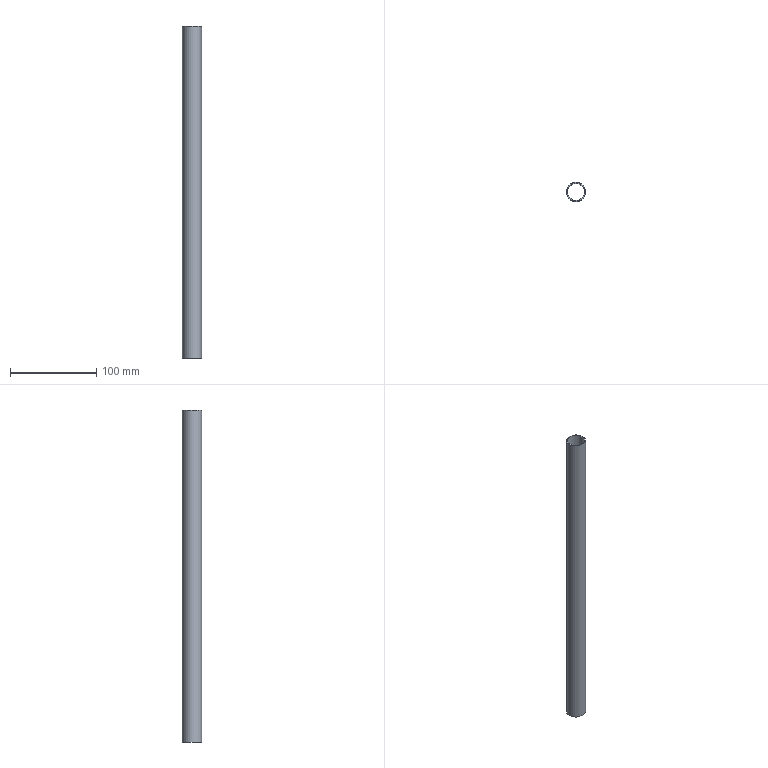Part | NX | features pipe belum expand 2 | 1 solid | 4 faces | box 22.2 x 22.2 x 385 mm | volume 30480 mm3 | cylinder 2 | plane 2 | commonest cylinder face diameters 19.8 x1 22.2 x1
STEP:
#1=CARTESIAN_POINT('',(9.9,0.,0.));
#2=VERTEX_POINT('',#1);
#3=CARTESIAN_POINT('',(0.,0.,0.));
#4=DIRECTION('',(0.,0.,1.));
#5=DIRECTION('',(1.,0.,0.));
#6=AXIS2_PLACEMENT_3D('',#3,#4,#5);
#7=CIRCLE('',#6,9.9);
#8=EDGE_CURVE('',#2,#2,#7,.F.);
#9=ORIENTED_EDGE('',*,*,#8,.F.);
#10=EDGE_LOOP('',(#9));
#11=FACE_BOUND('',#10,.T.);
#12=CARTESIAN_POINT('',(9.9,0.,-385.));
#13=VERTEX_POINT('',#12);
#14=CARTESIAN_POINT('',(0.,0.,-385.));
#15=DIRECTION('',(0.,0.,1.));
#16=DIRECTION('',(1.,0.,0.));
#17=AXIS2_PLACEMENT_3D('',#14,#15,#16);
#18=CIRCLE('',#17,9.9);
#19=EDGE_CURVE('',#13,#13,#18,.F.);
#20=ORIENTED_EDGE('',*,*,#19,.T.);
#21=EDGE_LOOP('',(#20));
#22=FACE_BOUND('',#21,.T.);
#23=CARTESIAN_POINT('',(0.,0.,-385.));
#24=DIRECTION('',(0.,0.,1.));
#25=DIRECTION('',(1.,0.,0.));
#26=AXIS2_PLACEMENT_3D('',#23,#24,#25);
#27=CYLINDRICAL_SURFACE('',#26,9.9);
#28=ADVANCED_FACE('',(#11,#22),#27,.F.);
#29=CARTESIAN_POINT('',(11.1,0.,-385.));
#30=VERTEX_POINT('',#29);
#31=CARTESIAN_POINT('',(0.,0.,-385.));
#32=DIRECTION('',(0.,0.,1.));
#33=DIRECTION('',(1.,0.,0.));
#34=AXIS2_PLACEMENT_3D('',#31,#32,#33);
#35=CIRCLE('',#34,11.1);
#36=EDGE_CURVE('',#30,#30,#35,.T.);
#37=ORIENTED_EDGE('',*,*,#36,.F.);
#38=EDGE_LOOP('',(#37));
#39=FACE_BOUND('',#38,.T.);
#40=ORIENTED_EDGE('',*,*,#19,.F.);
#41=EDGE_LOOP('',(#40));
#42=FACE_BOUND('',#41,.T.);
#43=CARTESIAN_POINT('',(0.,0.,-385.));
#44=DIRECTION('',(0.,0.,1.));
#45=DIRECTION('',(1.,0.,0.));
#46=AXIS2_PLACEMENT_3D('',#43,#44,#45);
#47=PLANE('',#46);
#48=ADVANCED_FACE('',(#39,#42),#47,.F.);
#49=CARTESIAN_POINT('',(11.1,0.,0.));
#50=VERTEX_POINT('',#49);
#51=CARTESIAN_POINT('',(0.,0.,0.));
#52=DIRECTION('',(0.,0.,1.));
#53=DIRECTION('',(1.,0.,0.));
#54=AXIS2_PLACEMENT_3D('',#51,#52,#53);
#55=CIRCLE('',#54,11.1);
#56=EDGE_CURVE('',#50,#50,#55,.F.);
#57=ORIENTED_EDGE('',*,*,#56,.F.);
#58=EDGE_LOOP('',(#57));
#59=FACE_BOUND('',#58,.T.);
#60=ORIENTED_EDGE('',*,*,#8,.T.);
#61=EDGE_LOOP('',(#60));
#62=FACE_BOUND('',#61,.T.);
#63=CARTESIAN_POINT('',(0.,0.,0.));
#64=DIRECTION('',(0.,0.,1.));
#65=DIRECTION('',(1.,0.,0.));
#66=AXIS2_PLACEMENT_3D('',#63,#64,#65);
#67=PLANE('',#66);
#68=ADVANCED_FACE('',(#59,#62),#67,.T.);
#69=ORIENTED_EDGE('',*,*,#56,.T.);
#70=EDGE_LOOP('',(#69));
#71=FACE_BOUND('',#70,.T.);
#72=ORIENTED_EDGE('',*,*,#36,.T.);
#73=EDGE_LOOP('',(#72));
#74=FACE_BOUND('',#73,.T.);
#75=CARTESIAN_POINT('',(0.,0.,-385.));
#76=DIRECTION('',(0.,0.,1.));
#77=DIRECTION('',(1.,0.,0.));
#78=AXIS2_PLACEMENT_3D('',#75,#76,#77);
#79=CYLINDRICAL_SURFACE('',#78,11.1);
#80=ADVANCED_FACE('',(#71,#74),#79,.T.);
#81=CLOSED_SHELL('',(#28,#48,#68,#80));
#82=MANIFOLD_SOLID_BREP('',#81);
#83=(LENGTH_UNIT()NAMED_UNIT(*)SI_UNIT(.MILLI.,.METRE.));
#84=UNCERTAINTY_MEASURE_WITH_UNIT(LENGTH_MEASURE(0.00001),#83,'','');
#85=(NAMED_UNIT(*)PLANE_ANGLE_UNIT()SI_UNIT($,.RADIAN.));
#86=(NAMED_UNIT(*)SI_UNIT($,.STERADIAN.)SOLID_ANGLE_UNIT());
#87=(GEOMETRIC_REPRESENTATION_CONTEXT(3)GLOBAL_UNCERTAINTY_ASSIGNED_CONTEXT((#84))GLOBAL_UNIT_ASSIGNED_CONTEXT((#83,#85,#86))REPRESENTATION_CONTEXT('',''));
#88=ADVANCED_BREP_SHAPE_REPRESENTATION('',(#82),#87);